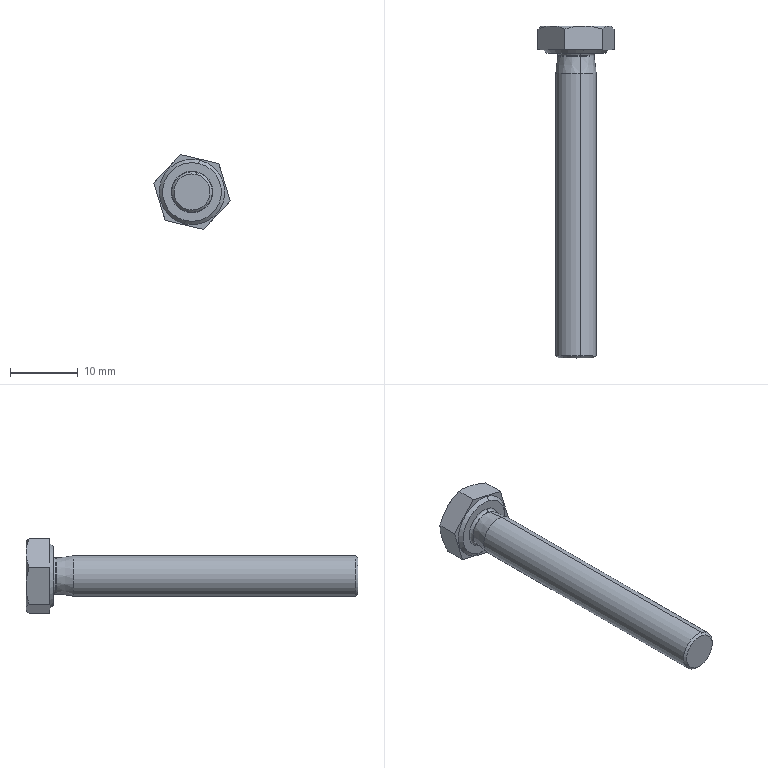Part | STEP file | Cut-Revolve 2-16 | 1 solid | 28 faces | box 11.242 x 49 x 11.054 mm | volume 1597 mm3 | cone 12 | plane 10 | torus 4 | cylinder 2 | commonest cylinder face diameters 6 x2
STEP:
#1=CARTESIAN_POINT('',(-1488.127,1719.714,2889.355));
#2=VERTEX_POINT('',#1);
#3=CARTESIAN_POINT('',(-1488.036,1720.114,2889.745));
#4=VERTEX_POINT('',#3);
#5=CARTESIAN_POINT('',(-1488.036,1719.714,2889.745));
#6=DIRECTION('',(0.9736,0.,-0.2284));
#7=DIRECTION('',(-0.2284,0.,-0.9736));
#8=AXIS2_PLACEMENT_3D('',#5,#6,#7);
#9=CIRCLE('',#8,0.4);
#10=EDGE_CURVE('',#2,#4,#9,.T.);
#11=ORIENTED_EDGE('',*,*,#10,.F.);
#12=CARTESIAN_POINT('',(-1489.349,1719.714,2884.146));
#13=VERTEX_POINT('',#12);
#14=CARTESIAN_POINT('',(-1488.738,1719.714,2886.751));
#15=DIRECTION('',(0.,1.,0.));
#16=DIRECTION('',(0.2284,0.,0.9736));
#17=AXIS2_PLACEMENT_3D('',#14,#15,#16);
#18=CIRCLE('',#17,2.675);
#19=EDGE_CURVE('',#2,#13,#18,.T.);
#20=ORIENTED_EDGE('',*,*,#19,.T.);
#21=CARTESIAN_POINT('',(-1489.441,1720.114,2883.757));
#22=VERTEX_POINT('',#21);
#23=CARTESIAN_POINT('',(-1489.441,1719.714,2883.757));
#24=DIRECTION('',(-0.9736,0.,0.2284));
#25=DIRECTION('',(0.2284,0.,0.9736));
#26=AXIS2_PLACEMENT_3D('',#23,#24,#25);
#27=CIRCLE('',#26,0.4);
#28=EDGE_CURVE('',#13,#22,#27,.T.);
#29=ORIENTED_EDGE('',*,*,#28,.T.);
#30=CARTESIAN_POINT('',(-1488.738,1720.114,2886.751));
#31=DIRECTION('',(0.,1.,0.));
#32=DIRECTION('',(0.2284,0.,0.9736));
#33=AXIS2_PLACEMENT_3D('',#30,#31,#32);
#34=CIRCLE('',#33,3.075);
#35=EDGE_CURVE('',#4,#22,#34,.T.);
#36=ORIENTED_EDGE('',*,*,#35,.F.);
#37=EDGE_LOOP('',(#11,#20,#29,#36));
#38=FACE_OUTER_BOUND('',#37,.T.);
#39=CARTESIAN_POINT('',(-1488.738,1719.714,2886.751));
#40=DIRECTION('',(0.,1.,0.));
#41=DIRECTION('',(-0.2284,0.,-0.9736));
#42=AXIS2_PLACEMENT_3D('',#39,#40,#41);
#43=TOROIDAL_SURFACE('',#42,3.075,0.4);
#44=ADVANCED_FACE('',(#38),#43,.F.);
#45=ORIENTED_EDGE('',*,*,#28,.F.);
#46=CARTESIAN_POINT('',(-1488.738,1719.714,2886.751));
#47=DIRECTION('',(0.,1.,0.));
#48=DIRECTION('',(0.2284,0.,0.9736));
#49=AXIS2_PLACEMENT_3D('',#46,#47,#48);
#50=CIRCLE('',#49,2.675);
#51=EDGE_CURVE('',#13,#2,#50,.T.);
#52=ORIENTED_EDGE('',*,*,#51,.T.);
#53=ORIENTED_EDGE('',*,*,#10,.T.);
#54=CARTESIAN_POINT('',(-1488.738,1720.114,2886.751));
#55=DIRECTION('',(0.,1.,0.));
#56=DIRECTION('',(0.2284,0.,0.9736));
#57=AXIS2_PLACEMENT_3D('',#54,#55,#56);
#58=CIRCLE('',#57,3.075);
#59=EDGE_CURVE('',#22,#4,#58,.T.);
#60=ORIENTED_EDGE('',*,*,#59,.F.);
#61=EDGE_LOOP('',(#45,#52,#53,#60));
#62=FACE_OUTER_BOUND('',#61,.T.);
#63=CARTESIAN_POINT('',(-1488.738,1719.714,2886.751));
#64=DIRECTION('',(0.,1.,0.));
#65=DIRECTION('',(-0.2284,0.,-0.9736));
#66=AXIS2_PLACEMENT_3D('',#63,#64,#65);
#67=TOROIDAL_SURFACE('',#66,3.075,0.4);
#68=ADVANCED_FACE('',(#62),#67,.F.);
#69=CARTESIAN_POINT('',(-1487.747,1720.114,2890.976));
#70=VERTEX_POINT('',#69);
#71=CARTESIAN_POINT('',(-1489.73,1720.114,2882.525));
#72=VERTEX_POINT('',#71);
#73=CARTESIAN_POINT('',(-1488.738,1720.114,2886.751));
#74=DIRECTION('',(0.,1.,0.));
#75=DIRECTION('',(0.2284,0.,0.9736));
#76=AXIS2_PLACEMENT_3D('',#73,#74,#75);
#77=CIRCLE('',#76,4.34);
#78=EDGE_CURVE('',#70,#72,#77,.T.);
#79=ORIENTED_EDGE('',*,*,#78,.T.);
#80=CARTESIAN_POINT('',(-1489.844,1720.614,2882.039));
#81=VERTEX_POINT('',#80);
#82=CARTESIAN_POINT('',(-1489.844,1720.614,2882.039));
#83=DIRECTION('',(-0.1615,0.7071,-0.6884));
#84=VECTOR('',#83,1000.);
#85=LINE('',#82,#84);
#86=EDGE_CURVE('',#72,#81,#85,.T.);
#87=ORIENTED_EDGE('',*,*,#86,.T.);
#88=CARTESIAN_POINT('',(-1487.633,1720.614,2891.463));
#89=VERTEX_POINT('',#88);
#90=CARTESIAN_POINT('',(-1488.738,1720.614,2886.751));
#91=DIRECTION('',(0.,1.,0.));
#92=DIRECTION('',(0.2284,0.,0.9736));
#93=AXIS2_PLACEMENT_3D('',#90,#91,#92);
#94=CIRCLE('',#93,4.84);
#95=EDGE_CURVE('',#89,#81,#94,.T.);
#96=ORIENTED_EDGE('',*,*,#95,.F.);
#97=CARTESIAN_POINT('',(-1487.633,1720.614,2891.463));
#98=DIRECTION('',(0.1615,0.7071,0.6884));
#99=VECTOR('',#98,1000.);
#100=LINE('',#97,#99);
#101=EDGE_CURVE('',#70,#89,#100,.T.);
#102=ORIENTED_EDGE('',*,*,#101,.F.);
#103=EDGE_LOOP('',(#79,#87,#96,#102));
#104=FACE_OUTER_BOUND('',#103,.T.);
#105=CARTESIAN_POINT('',(-1488.738,1720.614,2886.751));
#106=DIRECTION('',(0.,1.,0.));
#107=DIRECTION('',(-0.2284,0.,-0.9736));
#108=AXIS2_PLACEMENT_3D('',#105,#106,#107);
#109=CONICAL_SURFACE('',#108,4.84,0.7854);
#110=ADVANCED_FACE('',(#104),#109,.T.);
#111=CARTESIAN_POINT('',(-1489.347,1675.114,2884.155));
#112=VERTEX_POINT('',#111);
#113=CARTESIAN_POINT('',(-1488.129,1675.114,2889.347));
#114=VERTEX_POINT('',#113);
#115=CARTESIAN_POINT('',(-1488.738,1675.114,2886.751));
#116=DIRECTION('',(0.,-1.,0.));
#117=DIRECTION('',(0.2284,0.,0.9736));
#118=AXIS2_PLACEMENT_3D('',#115,#116,#117);
#119=CIRCLE('',#118,2.667);
#120=EDGE_CURVE('',#112,#114,#119,.T.);
#121=ORIENTED_EDGE('',*,*,#120,.F.);
#122=CARTESIAN_POINT('',(-1489.423,1675.448,2883.83));
#123=VERTEX_POINT('',#122);
#124=CARTESIAN_POINT('',(-1489.423,1675.448,2883.83));
#125=DIRECTION('',(-0.1615,0.7071,-0.6884));
#126=VECTOR('',#125,1000.);
#127=LINE('',#124,#126);
#128=EDGE_CURVE('',#112,#123,#127,.T.);
#129=ORIENTED_EDGE('',*,*,#128,.T.);
#130=CARTESIAN_POINT('',(-1488.053,1675.448,2889.671));
#131=VERTEX_POINT('',#130);
#132=CARTESIAN_POINT('',(-1488.738,1675.448,2886.751));
#133=DIRECTION('',(0.,1.,0.));
#134=DIRECTION('',(0.2284,0.,0.9736));
#135=AXIS2_PLACEMENT_3D('',#132,#133,#134);
#136=CIRCLE('',#135,3.);
#137=EDGE_CURVE('',#131,#123,#136,.T.);
#138=ORIENTED_EDGE('',*,*,#137,.F.);
#139=CARTESIAN_POINT('',(-1488.053,1675.448,2889.671));
#140=DIRECTION('',(0.1615,0.7071,0.6884));
#141=VECTOR('',#140,1000.);
#142=LINE('',#139,#141);
#143=EDGE_CURVE('',#114,#131,#142,.T.);
#144=ORIENTED_EDGE('',*,*,#143,.F.);
#145=EDGE_LOOP('',(#121,#129,#138,#144));
#146=FACE_OUTER_BOUND('',#145,.T.);
#147=CARTESIAN_POINT('',(-1488.738,1675.448,2886.751));
#148=DIRECTION('',(0.,1.,0.));
#149=DIRECTION('',(-0.2284,0.,-0.9736));
#150=AXIS2_PLACEMENT_3D('',#147,#148,#149);
#151=CONICAL_SURFACE('',#150,3.,0.7854);
#152=ADVANCED_FACE('',(#146),#151,.T.);
#153=ORIENTED_EDGE('',*,*,#51,.F.);
#154=CARTESIAN_POINT('',(-1489.35,1719.664,2884.143));
#155=VERTEX_POINT('',#154);
#156=CARTESIAN_POINT('',(-1489.441,1719.714,2883.757));
#157=DIRECTION('',(0.9736,0.,-0.2284));
#158=DIRECTION('',(0.2284,0.,0.9736));
#159=AXIS2_PLACEMENT_3D('',#156,#157,#158);
#160=CIRCLE('',#159,0.4);
#161=EDGE_CURVE('',#13,#155,#160,.T.);
#162=ORIENTED_EDGE('',*,*,#161,.T.);
#163=CARTESIAN_POINT('',(-1488.127,1719.664,2889.358));
#164=VERTEX_POINT('',#163);
#165=CARTESIAN_POINT('',(-1488.738,1719.664,2886.751));
#166=DIRECTION('',(0.,1.,0.));
#167=DIRECTION('',(0.2284,0.,0.9736));
#168=AXIS2_PLACEMENT_3D('',#165,#166,#167);
#169=CIRCLE('',#168,2.678);
#170=EDGE_CURVE('',#155,#164,#169,.T.);
#171=ORIENTED_EDGE('',*,*,#170,.T.);
#172=CARTESIAN_POINT('',(-1488.036,1719.714,2889.745));
#173=DIRECTION('',(-0.9736,0.,0.2284));
#174=DIRECTION('',(-0.2284,0.,-0.9736));
#175=AXIS2_PLACEMENT_3D('',#172,#173,#174);
#176=CIRCLE('',#175,0.4);
#177=EDGE_CURVE('',#2,#164,#176,.T.);
#178=ORIENTED_EDGE('',*,*,#177,.F.);
#179=EDGE_LOOP('',(#153,#162,#171,#178));
#180=FACE_OUTER_BOUND('',#179,.T.);
#181=CARTESIAN_POINT('',(-1488.738,1719.714,2886.751));
#182=DIRECTION('',(0.,1.,0.));
#183=DIRECTION('',(-0.2284,0.,-0.9736));
#184=AXIS2_PLACEMENT_3D('',#181,#182,#183);
#185=TOROIDAL_SURFACE('',#184,3.075,0.4);
#186=ADVANCED_FACE('',(#180),#185,.F.);
#187=ORIENTED_EDGE('',*,*,#137,.T.);
#188=CARTESIAN_POINT('',(-1489.423,1717.114,2883.83));
#189=VERTEX_POINT('',#188);
#190=CARTESIAN_POINT('',(-1489.423,1720.114,2883.83));
#191=DIRECTION('',(0.,1.,0.));
#192=VECTOR('',#191,1000.);
#193=LINE('',#190,#192);
#194=EDGE_CURVE('',#123,#189,#193,.T.);
#195=ORIENTED_EDGE('',*,*,#194,.T.);
#196=CARTESIAN_POINT('',(-1488.053,1717.114,2889.671));
#197=VERTEX_POINT('',#196);
#198=CARTESIAN_POINT('',(-1488.738,1717.114,2886.751));
#199=DIRECTION('',(0.,1.,0.));
#200=DIRECTION('',(0.2284,0.,0.9736));
#201=AXIS2_PLACEMENT_3D('',#198,#199,#200);
#202=CIRCLE('',#201,3.);
#203=EDGE_CURVE('',#197,#189,#202,.T.);
#204=ORIENTED_EDGE('',*,*,#203,.F.);
#205=CARTESIAN_POINT('',(-1488.053,1720.114,2889.671));
#206=DIRECTION('',(0.,1.,0.));
#207=VECTOR('',#206,1000.);
#208=LINE('',#205,#207);
#209=EDGE_CURVE('',#131,#197,#208,.T.);
#210=ORIENTED_EDGE('',*,*,#209,.F.);
#211=EDGE_LOOP('',(#187,#195,#204,#210));
#212=FACE_OUTER_BOUND('',#211,.T.);
#213=CARTESIAN_POINT('',(-1488.738,1720.114,2886.751));
#214=DIRECTION('',(0.,1.,0.));
#215=DIRECTION('',(-0.2284,0.,-0.9736));
#216=AXIS2_PLACEMENT_3D('',#213,#214,#215);
#217=CYLINDRICAL_SURFACE('',#216,3.);
#218=ADVANCED_FACE('',(#212),#217,.T.);
#219=CARTESIAN_POINT('',(-1488.738,1719.664,2886.751));
#220=DIRECTION('',(0.,1.,0.));
#221=DIRECTION('',(0.2284,0.,0.9736));
#222=AXIS2_PLACEMENT_3D('',#219,#220,#221);
#223=CIRCLE('',#222,2.678);
#224=EDGE_CURVE('',#164,#155,#223,.T.);
#225=ORIENTED_EDGE('',*,*,#224,.F.);
#226=CARTESIAN_POINT('',(-1488.053,1717.114,2889.671));
#227=DIRECTION('',(-0.02858,0.9921,-0.1218));
#228=VECTOR('',#227,1000.);
#229=LINE('',#226,#228);
#230=EDGE_CURVE('',#197,#164,#229,.T.);
#231=ORIENTED_EDGE('',*,*,#230,.F.);
#232=ORIENTED_EDGE('',*,*,#203,.T.);
#233=CARTESIAN_POINT('',(-1489.423,1717.114,2883.83));
#234=DIRECTION('',(0.02858,0.9921,0.1218));
#235=VECTOR('',#234,1000.);
#236=LINE('',#233,#235);
#237=EDGE_CURVE('',#189,#155,#236,.T.);
#238=ORIENTED_EDGE('',*,*,#237,.T.);
#239=EDGE_LOOP('',(#225,#231,#232,#238));
#240=FACE_OUTER_BOUND('',#239,.T.);
#241=CARTESIAN_POINT('',(-1488.738,1717.114,2886.751));
#242=DIRECTION('',(0.,-1.,0.));
#243=DIRECTION('',(0.2284,0.,0.9736));
#244=AXIS2_PLACEMENT_3D('',#241,#242,#243);
#245=CONICAL_SURFACE('',#244,3.,0.1255);
#246=ADVANCED_FACE('',(#240),#245,.T.);
#247=ORIENTED_EDGE('',*,*,#35,.T.);
#248=ORIENTED_EDGE('',*,*,#59,.T.);
#249=EDGE_LOOP('',(#247,#248));
#250=FACE_BOUND('',#249,.T.);
#251=ORIENTED_EDGE('',*,*,#78,.F.);
#252=CARTESIAN_POINT('',(-1488.738,1720.114,2886.751));
#253=DIRECTION('',(0.,1.,0.));
#254=DIRECTION('',(0.2284,0.,0.9736));
#255=AXIS2_PLACEMENT_3D('',#252,#253,#254);
#256=CIRCLE('',#255,4.34);
#257=EDGE_CURVE('',#72,#70,#256,.T.);
#258=ORIENTED_EDGE('',*,*,#257,.F.);
#259=EDGE_LOOP('',(#251,#258));
#260=FACE_OUTER_BOUND('',#259,.T.);
#261=CARTESIAN_POINT('',(-1487.07,1720.114,2881.224));
#262=DIRECTION('',(0.,-1.,0.));
#263=DIRECTION('',(0.2284,0.,0.9736));
#264=AXIS2_PLACEMENT_3D('',#261,#262,#263);
#265=PLANE('',#264);
#266=ADVANCED_FACE('',(#250,#260),#265,.T.);
#267=ORIENTED_EDGE('',*,*,#230,.T.);
#268=ORIENTED_EDGE('',*,*,#170,.F.);
#269=ORIENTED_EDGE('',*,*,#237,.F.);
#270=CARTESIAN_POINT('',(-1488.738,1717.114,2886.751));
#271=DIRECTION('',(0.,1.,0.));
#272=DIRECTION('',(0.2284,0.,0.9736));
#273=AXIS2_PLACEMENT_3D('',#270,#271,#272);
#274=CIRCLE('',#273,3.);
#275=EDGE_CURVE('',#189,#197,#274,.T.);
#276=ORIENTED_EDGE('',*,*,#275,.T.);
#277=EDGE_LOOP('',(#267,#268,#269,#276));
#278=FACE_OUTER_BOUND('',#277,.T.);
#279=CARTESIAN_POINT('',(-1488.738,1717.114,2886.751));
#280=DIRECTION('',(0.,-1.,0.));
#281=DIRECTION('',(0.2284,0.,0.9736));
#282=AXIS2_PLACEMENT_3D('',#279,#280,#281);
#283=CONICAL_SURFACE('',#282,3.,0.1255);
#284=ADVANCED_FACE('',(#278),#283,.T.);
#285=ORIENTED_EDGE('',*,*,#194,.F.);
#286=CARTESIAN_POINT('',(-1488.738,1675.448,2886.751));
#287=DIRECTION('',(0.,1.,0.));
#288=DIRECTION('',(0.2284,0.,0.9736));
#289=AXIS2_PLACEMENT_3D('',#286,#287,#288);
#290=CIRCLE('',#289,3.);
#291=EDGE_CURVE('',#123,#131,#290,.T.);
#292=ORIENTED_EDGE('',*,*,#291,.T.);
#293=ORIENTED_EDGE('',*,*,#209,.T.);
#294=ORIENTED_EDGE('',*,*,#275,.F.);
#295=EDGE_LOOP('',(#285,#292,#293,#294));
#296=FACE_OUTER_BOUND('',#295,.T.);
#297=CARTESIAN_POINT('',(-1488.738,1720.114,2886.751));
#298=DIRECTION('',(0.,1.,0.));
#299=DIRECTION('',(-0.2284,0.,-0.9736));
#300=AXIS2_PLACEMENT_3D('',#297,#298,#299);
#301=CYLINDRICAL_SURFACE('',#300,3.);
#302=ADVANCED_FACE('',(#296),#301,.T.);
#303=CARTESIAN_POINT('',(-1488.738,1675.114,2886.751));
#304=DIRECTION('',(0.,-1.,0.));
#305=DIRECTION('',(0.2284,0.,0.9736));
#306=AXIS2_PLACEMENT_3D('',#303,#304,#305);
#307=CIRCLE('',#306,2.667);
#308=EDGE_CURVE('',#114,#112,#307,.T.);
#309=ORIENTED_EDGE('',*,*,#308,.T.);
#310=ORIENTED_EDGE('',*,*,#120,.T.);
#311=EDGE_LOOP('',(#309,#310));
#312=FACE_OUTER_BOUND('',#311,.T.);
#313=CARTESIAN_POINT('',(-1485.818,1675.114,2886.065));
#314=DIRECTION('',(0.,1.,0.));
#315=DIRECTION('',(-0.2284,0.,-0.9736));
#316=AXIS2_PLACEMENT_3D('',#313,#314,#315);
#317=PLANE('',#316);
#318=ADVANCED_FACE('',(#312),#317,.F.);
#319=ORIENTED_EDGE('',*,*,#19,.F.);
#320=ORIENTED_EDGE('',*,*,#177,.T.);
#321=ORIENTED_EDGE('',*,*,#224,.T.);
#322=ORIENTED_EDGE('',*,*,#161,.F.);
#323=EDGE_LOOP('',(#319,#320,#321,#322));
#324=FACE_OUTER_BOUND('',#323,.T.);
#325=CARTESIAN_POINT('',(-1488.738,1719.714,2886.751));
#326=DIRECTION('',(0.,1.,0.));
#327=DIRECTION('',(-0.2284,0.,-0.9736));
#328=AXIS2_PLACEMENT_3D('',#325,#326,#327);
#329=TOROIDAL_SURFACE('',#328,3.075,0.4);
#330=ADVANCED_FACE('',(#324),#329,.F.);
#331=ORIENTED_EDGE('',*,*,#128,.F.);
#332=ORIENTED_EDGE('',*,*,#308,.F.);
#333=ORIENTED_EDGE('',*,*,#143,.T.);
#334=ORIENTED_EDGE('',*,*,#291,.F.);
#335=EDGE_LOOP('',(#331,#332,#333,#334));
#336=FACE_OUTER_BOUND('',#335,.T.);
#337=CARTESIAN_POINT('',(-1488.738,1675.448,2886.751));
#338=DIRECTION('',(0.,1.,0.));
#339=DIRECTION('',(-0.2284,0.,-0.9736));
#340=AXIS2_PLACEMENT_3D('',#337,#338,#339);
#341=CONICAL_SURFACE('',#340,3.,0.7854);
#342=ADVANCED_FACE('',(#336),#341,.T.);
#343=ORIENTED_EDGE('',*,*,#95,.T.);
#344=CARTESIAN_POINT('',(-1488.738,1720.614,2886.751));
#345=DIRECTION('',(0.,1.,0.));
#346=DIRECTION('',(0.2284,0.,0.9736));
#347=AXIS2_PLACEMENT_3D('',#344,#345,#346);
#348=CIRCLE('',#347,4.84);
#349=EDGE_CURVE('',#81,#89,#348,.T.);
#350=ORIENTED_EDGE('',*,*,#349,.T.);
#351=EDGE_LOOP('',(#343,#350));
#352=FACE_BOUND('',#351,.T.);
#353=CARTESIAN_POINT('',(-1492.691,1720.614,2882.542));
#354=VERTEX_POINT('',#353);
#355=CARTESIAN_POINT('',(-1487.07,1720.614,2881.224));
#356=VERTEX_POINT('',#355);
#357=CARTESIAN_POINT('',(-1492.691,1720.614,2882.542));
#358=DIRECTION('',(0.9736,0.,-0.2284));
#359=VECTOR('',#358,1000.);
#360=LINE('',#357,#359);
#361=EDGE_CURVE('',#354,#356,#360,.T.);
#362=ORIENTED_EDGE('',*,*,#361,.T.);
#363=CARTESIAN_POINT('',(-1483.117,1720.614,2885.432));
#364=VERTEX_POINT('',#363);
#365=CARTESIAN_POINT('',(-1487.07,1720.614,2881.224));
#366=DIRECTION('',(0.6846,0.,0.7289));
#367=VECTOR('',#366,1000.);
#368=LINE('',#365,#367);
#369=EDGE_CURVE('',#356,#364,#368,.T.);
#370=ORIENTED_EDGE('',*,*,#369,.T.);
#371=CARTESIAN_POINT('',(-1484.786,1720.614,2890.959));
#372=VERTEX_POINT('',#371);
#373=CARTESIAN_POINT('',(-1483.117,1720.614,2885.432));
#374=DIRECTION('',(-0.289,0.,0.9573));
#375=VECTOR('',#374,1000.);
#376=LINE('',#373,#375);
#377=EDGE_CURVE('',#364,#372,#376,.T.);
#378=ORIENTED_EDGE('',*,*,#377,.T.);
#379=CARTESIAN_POINT('',(-1490.407,1720.614,2892.278));
#380=VERTEX_POINT('',#379);
#381=CARTESIAN_POINT('',(-1484.786,1720.614,2890.959));
#382=DIRECTION('',(-0.9736,0.,0.2284));
#383=VECTOR('',#382,1000.);
#384=LINE('',#381,#383);
#385=EDGE_CURVE('',#372,#380,#384,.T.);
#386=ORIENTED_EDGE('',*,*,#385,.T.);
#387=CARTESIAN_POINT('',(-1494.359,1720.614,2888.069));
#388=VERTEX_POINT('',#387);
#389=CARTESIAN_POINT('',(-1490.407,1720.614,2892.278));
#390=DIRECTION('',(-0.6846,0.,-0.7289));
#391=VECTOR('',#390,1000.);
#392=LINE('',#389,#391);
#393=EDGE_CURVE('',#380,#388,#392,.T.);
#394=ORIENTED_EDGE('',*,*,#393,.T.);
#395=CARTESIAN_POINT('',(-1494.359,1720.614,2888.069));
#396=DIRECTION('',(0.289,0.,-0.9573));
#397=VECTOR('',#396,1000.);
#398=LINE('',#395,#397);
#399=EDGE_CURVE('',#388,#354,#398,.T.);
#400=ORIENTED_EDGE('',*,*,#399,.T.);
#401=EDGE_LOOP('',(#362,#370,#378,#386,#394,#400));
#402=FACE_OUTER_BOUND('',#401,.T.);
#403=CARTESIAN_POINT('',(-1493.45,1720.614,2887.856));
#404=DIRECTION('',(0.,-1.,0.));
#405=DIRECTION('',(0.2284,0.,0.9736));
#406=AXIS2_PLACEMENT_3D('',#403,#404,#405);
#407=PLANE('',#406);
#408=ADVANCED_FACE('',(#352,#402),#407,.T.);
#409=ORIENTED_EDGE('',*,*,#86,.F.);
#410=ORIENTED_EDGE('',*,*,#257,.T.);
#411=ORIENTED_EDGE('',*,*,#101,.T.);
#412=ORIENTED_EDGE('',*,*,#349,.F.);
#413=EDGE_LOOP('',(#409,#410,#411,#412));
#414=FACE_OUTER_BOUND('',#413,.T.);
#415=CARTESIAN_POINT('',(-1488.738,1720.614,2886.751));
#416=DIRECTION('',(0.,1.,0.));
#417=DIRECTION('',(-0.2284,0.,-0.9736));
#418=AXIS2_PLACEMENT_3D('',#415,#416,#417);
#419=CONICAL_SURFACE('',#418,4.84,0.7854);
#420=ADVANCED_FACE('',(#414),#419,.T.);
#421=CARTESIAN_POINT('',(-1489.88,1724.114,2881.883));
#422=VERTEX_POINT('',#421);
#423=CARTESIAN_POINT('',(-1485.094,1724.114,2883.328));
#424=VERTEX_POINT('',#423);
#425=CARTESIAN_POINT('',(-1488.738,1724.114,2886.751));
#426=DIRECTION('',(0.,-1.,0.));
#427=DIRECTION('',(-0.2284,0.,-0.9736));
#428=AXIS2_PLACEMENT_3D('',#425,#426,#427);
#429=CIRCLE('',#428,5.);
#430=EDGE_CURVE('',#422,#424,#429,.T.);
#431=ORIENTED_EDGE('',*,*,#430,.F.);
#432=CARTESIAN_POINT('',(-1493.525,1724.114,2885.306));
#433=VERTEX_POINT('',#432);
#434=CARTESIAN_POINT('',(-1488.738,1724.114,2886.751));
#435=DIRECTION('',(0.,-1.,0.));
#436=DIRECTION('',(-0.2284,0.,-0.9736));
#437=AXIS2_PLACEMENT_3D('',#434,#435,#436);
#438=CIRCLE('',#437,5.);
#439=EDGE_CURVE('',#433,#422,#438,.T.);
#440=ORIENTED_EDGE('',*,*,#439,.F.);
#441=CARTESIAN_POINT('',(-1492.383,1724.114,2890.174));
#442=VERTEX_POINT('',#441);
#443=CARTESIAN_POINT('',(-1488.738,1724.114,2886.751));
#444=DIRECTION('',(0.,-1.,0.));
#445=DIRECTION('',(-0.2284,0.,-0.9736));
#446=AXIS2_PLACEMENT_3D('',#443,#444,#445);
#447=CIRCLE('',#446,5.);
#448=EDGE_CURVE('',#442,#433,#447,.T.);
#449=ORIENTED_EDGE('',*,*,#448,.F.);
#450=CARTESIAN_POINT('',(-1487.596,1724.114,2891.619));
#451=VERTEX_POINT('',#450);
#452=CARTESIAN_POINT('',(-1488.738,1724.114,2886.751));
#453=DIRECTION('',(0.,-1.,0.));
#454=DIRECTION('',(-0.2284,0.,-0.9736));
#455=AXIS2_PLACEMENT_3D('',#452,#453,#454);
#456=CIRCLE('',#455,5.);
#457=EDGE_CURVE('',#451,#442,#456,.T.);
#458=ORIENTED_EDGE('',*,*,#457,.F.);
#459=CARTESIAN_POINT('',(-1483.952,1724.114,2888.196));
#460=VERTEX_POINT('',#459);
#461=CARTESIAN_POINT('',(-1488.738,1724.114,2886.751));
#462=DIRECTION('',(0.,1.,0.));
#463=DIRECTION('',(0.2284,0.,0.9736));
#464=AXIS2_PLACEMENT_3D('',#461,#462,#463);
#465=CIRCLE('',#464,5.);
#466=EDGE_CURVE('',#451,#460,#465,.T.);
#467=ORIENTED_EDGE('',*,*,#466,.T.);
#468=CARTESIAN_POINT('',(-1488.738,1724.114,2886.751));
#469=DIRECTION('',(0.,-1.,0.));
#470=DIRECTION('',(-0.2284,0.,-0.9736));
#471=AXIS2_PLACEMENT_3D('',#468,#469,#470);
#472=CIRCLE('',#471,5.);
#473=EDGE_CURVE('',#424,#460,#472,.T.);
#474=ORIENTED_EDGE('',*,*,#473,.F.);
#475=EDGE_LOOP('',(#431,#440,#449,#458,#467,#474));
#476=FACE_OUTER_BOUND('',#475,.T.);
#477=CARTESIAN_POINT('',(-1487.07,1724.114,2881.224));
#478=DIRECTION('',(0.,-1.,0.));
#479=DIRECTION('',(0.2284,0.,0.9736));
#480=AXIS2_PLACEMENT_3D('',#477,#478,#479);
#481=PLANE('',#480);
#482=ADVANCED_FACE('',(#476),#481,.F.);
#483=CARTESIAN_POINT('',(-1487.07,1723.668,2881.224));
#484=VERTEX_POINT('',#483);
#485=CARTESIAN_POINT('',(-1485.094,1724.114,2883.328));
#486=CARTESIAN_POINT('',(-1485.768,1724.114,2882.61));
#487=CARTESIAN_POINT('',(-1486.424,1723.94,2881.911));
#488=CARTESIAN_POINT('',(-1487.07,1723.668,2881.224));
#489=B_SPLINE_CURVE_WITH_KNOTS('',3,(#485,#486,#487,#488),.UNSPECIFIED.,.F.,.F.,(4,4),(0.,0.002921),.UNSPECIFIED.);
#490=EDGE_CURVE('',#424,#484,#489,.T.);
#491=ORIENTED_EDGE('',*,*,#490,.T.);
#492=CARTESIAN_POINT('',(-1487.07,1723.668,2881.224));
#493=CARTESIAN_POINT('',(-1487.988,1723.94,2881.439));
#494=CARTESIAN_POINT('',(-1488.921,1724.114,2881.658));
#495=CARTESIAN_POINT('',(-1489.88,1724.114,2881.883));
#496=B_SPLINE_CURVE_WITH_KNOTS('',3,(#492,#493,#494,#495),.UNSPECIFIED.,.F.,.F.,(4,4),(0.,0.002921),.UNSPECIFIED.);
#497=EDGE_CURVE('',#484,#422,#496,.T.);
#498=ORIENTED_EDGE('',*,*,#497,.T.);
#499=ORIENTED_EDGE('',*,*,#430,.T.);
#500=EDGE_LOOP('',(#491,#498,#499));
#501=FACE_OUTER_BOUND('',#500,.T.);
#502=CARTESIAN_POINT('',(-1488.738,1724.114,2886.751));
#503=DIRECTION('',(0.,-1.,0.));
#504=DIRECTION('',(-0.2284,0.,-0.9736));
#505=AXIS2_PLACEMENT_3D('',#502,#503,#504);
#506=CONICAL_SURFACE('',#505,5.,1.047);
#507=ADVANCED_FACE('',(#501),#506,.T.);
#508=CARTESIAN_POINT('',(-1483.117,1723.668,2885.432));
#509=VERTEX_POINT('',#508);
#510=CARTESIAN_POINT('',(-1483.952,1724.114,2888.196));
#511=CARTESIAN_POINT('',(-1483.667,1724.114,2887.252));
#512=CARTESIAN_POINT('',(-1483.39,1723.94,2886.335));
#513=CARTESIAN_POINT('',(-1483.117,1723.668,2885.432));
#514=B_SPLINE_CURVE_WITH_KNOTS('',3,(#510,#511,#512,#513),.UNSPECIFIED.,.F.,.F.,(4,4),(0.,0.002921),.UNSPECIFIED.);
#515=EDGE_CURVE('',#460,#509,#514,.T.);
#516=ORIENTED_EDGE('',*,*,#515,.T.);
#517=CARTESIAN_POINT('',(-1483.117,1723.668,2885.432));
#518=CARTESIAN_POINT('',(-1483.763,1723.94,2884.745));
#519=CARTESIAN_POINT('',(-1484.419,1724.114,2884.046));
#520=CARTESIAN_POINT('',(-1485.094,1724.114,2883.328));
#521=B_SPLINE_CURVE_WITH_KNOTS('',3,(#517,#518,#519,#520),.UNSPECIFIED.,.F.,.F.,(4,4),(0.,0.002921),.UNSPECIFIED.);
#522=EDGE_CURVE('',#509,#424,#521,.T.);
#523=ORIENTED_EDGE('',*,*,#522,.T.);
#524=ORIENTED_EDGE('',*,*,#473,.T.);
#525=EDGE_LOOP('',(#516,#523,#524));
#526=FACE_OUTER_BOUND('',#525,.T.);
#527=CARTESIAN_POINT('',(-1488.738,1724.114,2886.751));
#528=DIRECTION('',(0.,-1.,0.));
#529=DIRECTION('',(-0.2284,0.,-0.9736));
#530=AXIS2_PLACEMENT_3D('',#527,#528,#529);
#531=CONICAL_SURFACE('',#530,5.,1.047);
#532=ADVANCED_FACE('',(#526),#531,.T.);
#533=CARTESIAN_POINT('',(-1484.786,1723.668,2890.959));
#534=VERTEX_POINT('',#533);
#535=CARTESIAN_POINT('',(-1484.786,1723.668,2890.959));
#536=CARTESIAN_POINT('',(-1484.513,1723.94,2890.056));
#537=CARTESIAN_POINT('',(-1484.236,1724.114,2889.139));
#538=CARTESIAN_POINT('',(-1483.952,1724.114,2888.196));
#539=B_SPLINE_CURVE_WITH_KNOTS('',3,(#535,#536,#537,#538),.UNSPECIFIED.,.F.,.F.,(4,4),(0.,0.002921),.UNSPECIFIED.);
#540=EDGE_CURVE('',#534,#460,#539,.T.);
#541=ORIENTED_EDGE('',*,*,#540,.T.);
#542=ORIENTED_EDGE('',*,*,#466,.F.);
#543=CARTESIAN_POINT('',(-1487.596,1724.114,2891.619));
#544=CARTESIAN_POINT('',(-1486.637,1724.114,2891.393));
#545=CARTESIAN_POINT('',(-1485.704,1723.94,2891.175));
#546=CARTESIAN_POINT('',(-1484.786,1723.668,2890.959));
#547=B_SPLINE_CURVE_WITH_KNOTS('',3,(#543,#544,#545,#546),.UNSPECIFIED.,.F.,.F.,(4,4),(0.,0.002921),.UNSPECIFIED.);
#548=EDGE_CURVE('',#451,#534,#547,.T.);
#549=ORIENTED_EDGE('',*,*,#548,.T.);
#550=EDGE_LOOP('',(#541,#542,#549));
#551=FACE_OUTER_BOUND('',#550,.T.);
#552=CARTESIAN_POINT('',(-1488.738,1724.114,2886.751));
#553=DIRECTION('',(0.,-1.,0.));
#554=DIRECTION('',(-0.2284,0.,-0.9736));
#555=AXIS2_PLACEMENT_3D('',#552,#553,#554);
#556=CONICAL_SURFACE('',#555,5.,1.047);
#557=ADVANCED_FACE('',(#551),#556,.T.);
#558=CARTESIAN_POINT('',(-1490.407,1723.668,2892.278));
#559=VERTEX_POINT('',#558);
#560=CARTESIAN_POINT('',(-1490.407,1723.668,2892.278));
#561=CARTESIAN_POINT('',(-1489.488,1723.94,2892.062));
#562=CARTESIAN_POINT('',(-1488.555,1724.114,2891.844));
#563=CARTESIAN_POINT('',(-1487.596,1724.114,2891.619));
#564=B_SPLINE_CURVE_WITH_KNOTS('',3,(#560,#561,#562,#563),.UNSPECIFIED.,.F.,.F.,(4,4),(0.,0.002921),.UNSPECIFIED.);
#565=EDGE_CURVE('',#559,#451,#564,.T.);
#566=ORIENTED_EDGE('',*,*,#565,.T.);
#567=ORIENTED_EDGE('',*,*,#457,.T.);
#568=CARTESIAN_POINT('',(-1492.383,1724.114,2890.174));
#569=CARTESIAN_POINT('',(-1491.708,1724.114,2890.892));
#570=CARTESIAN_POINT('',(-1491.052,1723.94,2891.59));
#571=CARTESIAN_POINT('',(-1490.407,1723.668,2892.278));
#572=B_SPLINE_CURVE_WITH_KNOTS('',3,(#568,#569,#570,#571),.UNSPECIFIED.,.F.,.F.,(4,4),(0.,0.002921),.UNSPECIFIED.);
#573=EDGE_CURVE('',#442,#559,#572,.T.);
#574=ORIENTED_EDGE('',*,*,#573,.T.);
#575=EDGE_LOOP('',(#566,#567,#574));
#576=FACE_OUTER_BOUND('',#575,.T.);
#577=CARTESIAN_POINT('',(-1488.738,1724.114,2886.751));
#578=DIRECTION('',(0.,-1.,0.));
#579=DIRECTION('',(-0.2284,0.,-0.9736));
#580=AXIS2_PLACEMENT_3D('',#577,#578,#579);
#581=CONICAL_SURFACE('',#580,5.,1.047);
#582=ADVANCED_FACE('',(#576),#581,.T.);
#583=CARTESIAN_POINT('',(-1492.691,1723.668,2882.542));
#584=VERTEX_POINT('',#583);
#585=CARTESIAN_POINT('',(-1489.88,1724.114,2881.883));
#586=CARTESIAN_POINT('',(-1490.84,1724.114,2882.108));
#587=CARTESIAN_POINT('',(-1491.773,1723.94,2882.327));
#588=CARTESIAN_POINT('',(-1492.691,1723.668,2882.542));
#589=B_SPLINE_CURVE_WITH_KNOTS('',3,(#585,#586,#587,#588),.UNSPECIFIED.,.F.,.F.,(4,4),(0.,0.002921),.UNSPECIFIED.);
#590=EDGE_CURVE('',#422,#584,#589,.T.);
#591=ORIENTED_EDGE('',*,*,#590,.T.);
#592=CARTESIAN_POINT('',(-1492.691,1723.668,2882.542));
#593=CARTESIAN_POINT('',(-1492.963,1723.94,2883.445));
#594=CARTESIAN_POINT('',(-1493.24,1724.114,2884.363));
#595=CARTESIAN_POINT('',(-1493.525,1724.114,2885.306));
#596=B_SPLINE_CURVE_WITH_KNOTS('',3,(#592,#593,#594,#595),.UNSPECIFIED.,.F.,.F.,(4,4),(0.,0.002921),.UNSPECIFIED.);
#597=EDGE_CURVE('',#584,#433,#596,.T.);
#598=ORIENTED_EDGE('',*,*,#597,.T.);
#599=ORIENTED_EDGE('',*,*,#439,.T.);
#600=EDGE_LOOP('',(#591,#598,#599));
#601=FACE_OUTER_BOUND('',#600,.T.);
#602=CARTESIAN_POINT('',(-1488.738,1724.114,2886.751));
#603=DIRECTION('',(0.,-1.,0.));
#604=DIRECTION('',(-0.2284,0.,-0.9736));
#605=AXIS2_PLACEMENT_3D('',#602,#603,#604);
#606=CONICAL_SURFACE('',#605,5.,1.047);
#607=ADVANCED_FACE('',(#601),#606,.T.);
#608=CARTESIAN_POINT('',(-1494.359,1723.668,2888.069));
#609=VERTEX_POINT('',#608);
#610=CARTESIAN_POINT('',(-1494.359,1723.668,2888.069));
#611=CARTESIAN_POINT('',(-1493.713,1723.94,2888.757));
#612=CARTESIAN_POINT('',(-1493.057,1724.114,2889.455));
#613=CARTESIAN_POINT('',(-1492.383,1724.114,2890.174));
#614=B_SPLINE_CURVE_WITH_KNOTS('',3,(#610,#611,#612,#613),.UNSPECIFIED.,.F.,.F.,(4,4),(0.,0.002921),.UNSPECIFIED.);
#615=EDGE_CURVE('',#609,#442,#614,.T.);
#616=ORIENTED_EDGE('',*,*,#615,.T.);
#617=ORIENTED_EDGE('',*,*,#448,.T.);
#618=CARTESIAN_POINT('',(-1493.525,1724.114,2885.306));
#619=CARTESIAN_POINT('',(-1493.81,1724.114,2886.249));
#620=CARTESIAN_POINT('',(-1494.087,1723.94,2887.166));
#621=CARTESIAN_POINT('',(-1494.359,1723.668,2888.069));
#622=B_SPLINE_CURVE_WITH_KNOTS('',3,(#618,#619,#620,#621),.UNSPECIFIED.,.F.,.F.,(4,4),(0.,0.002921),.UNSPECIFIED.);
#623=EDGE_CURVE('',#433,#609,#622,.T.);
#624=ORIENTED_EDGE('',*,*,#623,.T.);
#625=EDGE_LOOP('',(#616,#617,#624));
#626=FACE_OUTER_BOUND('',#625,.T.);
#627=CARTESIAN_POINT('',(-1488.738,1724.114,2886.751));
#628=DIRECTION('',(0.,-1.,0.));
#629=DIRECTION('',(-0.2284,0.,-0.9736));
#630=AXIS2_PLACEMENT_3D('',#627,#628,#629);
#631=CONICAL_SURFACE('',#630,5.,1.047);
#632=ADVANCED_FACE('',(#626),#631,.T.);
#633=ORIENTED_EDGE('',*,*,#399,.F.);
#634=CARTESIAN_POINT('',(-1494.359,1720.114,2888.069));
#635=DIRECTION('',(0.,1.,0.));
#636=VECTOR('',#635,1000.);
#637=LINE('',#634,#636);
#638=EDGE_CURVE('',#388,#609,#637,.T.);
#639=ORIENTED_EDGE('',*,*,#638,.T.);
#640=ORIENTED_EDGE('',*,*,#623,.F.);
#641=ORIENTED_EDGE('',*,*,#597,.F.);
#642=CARTESIAN_POINT('',(-1492.691,1720.114,2882.542));
#643=DIRECTION('',(0.,1.,0.));
#644=VECTOR('',#643,1000.);
#645=LINE('',#642,#644);
#646=EDGE_CURVE('',#354,#584,#645,.T.);
#647=ORIENTED_EDGE('',*,*,#646,.F.);
#648=EDGE_LOOP('',(#633,#639,#640,#641,#647));
#649=FACE_OUTER_BOUND('',#648,.T.);
#650=CARTESIAN_POINT('',(-1494.359,1720.114,2888.069));
#651=DIRECTION('',(0.9573,0.,0.289));
#652=DIRECTION('',(0.289,0.,-0.9573));
#653=AXIS2_PLACEMENT_3D('',#650,#651,#652);
#654=PLANE('',#653);
#655=ADVANCED_FACE('',(#649),#654,.F.);
#656=ORIENTED_EDGE('',*,*,#393,.F.);
#657=CARTESIAN_POINT('',(-1490.407,1720.114,2892.278));
#658=DIRECTION('',(0.,1.,0.));
#659=VECTOR('',#658,1000.);
#660=LINE('',#657,#659);
#661=EDGE_CURVE('',#380,#559,#660,.T.);
#662=ORIENTED_EDGE('',*,*,#661,.T.);
#663=ORIENTED_EDGE('',*,*,#573,.F.);
#664=ORIENTED_EDGE('',*,*,#615,.F.);
#665=ORIENTED_EDGE('',*,*,#638,.F.);
#666=EDGE_LOOP('',(#656,#662,#663,#664,#665));
#667=FACE_OUTER_BOUND('',#666,.T.);
#668=CARTESIAN_POINT('',(-1490.407,1720.114,2892.278));
#669=DIRECTION('',(0.7289,0.,-0.6846));
#670=DIRECTION('',(-0.6846,0.,-0.7289));
#671=AXIS2_PLACEMENT_3D('',#668,#669,#670);
#672=PLANE('',#671);
#673=ADVANCED_FACE('',(#667),#672,.F.);
#674=ORIENTED_EDGE('',*,*,#385,.F.);
#675=CARTESIAN_POINT('',(-1484.786,1720.114,2890.959));
#676=DIRECTION('',(0.,1.,0.));
#677=VECTOR('',#676,1000.);
#678=LINE('',#675,#677);
#679=EDGE_CURVE('',#372,#534,#678,.T.);
#680=ORIENTED_EDGE('',*,*,#679,.T.);
#681=ORIENTED_EDGE('',*,*,#548,.F.);
#682=ORIENTED_EDGE('',*,*,#565,.F.);
#683=ORIENTED_EDGE('',*,*,#661,.F.);
#684=EDGE_LOOP('',(#674,#680,#681,#682,#683));
#685=FACE_OUTER_BOUND('',#684,.T.);
#686=CARTESIAN_POINT('',(-1484.786,1720.114,2890.959));
#687=DIRECTION('',(-0.2284,0.,-0.9736));
#688=DIRECTION('',(0.,-1.,0.));
#689=AXIS2_PLACEMENT_3D('',#686,#687,#688);
#690=PLANE('',#689);
#691=ADVANCED_FACE('',(#685),#690,.F.);
#692=ORIENTED_EDGE('',*,*,#377,.F.);
#693=CARTESIAN_POINT('',(-1483.117,1720.114,2885.432));
#694=DIRECTION('',(0.,1.,0.));
#695=VECTOR('',#694,1000.);
#696=LINE('',#693,#695);
#697=EDGE_CURVE('',#364,#509,#696,.T.);
#698=ORIENTED_EDGE('',*,*,#697,.T.);
#699=ORIENTED_EDGE('',*,*,#515,.F.);
#700=ORIENTED_EDGE('',*,*,#540,.F.);
#701=ORIENTED_EDGE('',*,*,#679,.F.);
#702=EDGE_LOOP('',(#692,#698,#699,#700,#701));
#703=FACE_OUTER_BOUND('',#702,.T.);
#704=CARTESIAN_POINT('',(-1483.117,1720.114,2885.432));
#705=DIRECTION('',(-0.9573,0.,-0.289));
#706=DIRECTION('',(-0.289,0.,0.9573));
#707=AXIS2_PLACEMENT_3D('',#704,#705,#706);
#708=PLANE('',#707);
#709=ADVANCED_FACE('',(#703),#708,.F.);
#710=ORIENTED_EDGE('',*,*,#369,.F.);
#711=CARTESIAN_POINT('',(-1487.07,1720.114,2881.224));
#712=DIRECTION('',(0.,1.,0.));
#713=VECTOR('',#712,1000.);
#714=LINE('',#711,#713);
#715=EDGE_CURVE('',#356,#484,#714,.T.);
#716=ORIENTED_EDGE('',*,*,#715,.T.);
#717=ORIENTED_EDGE('',*,*,#490,.F.);
#718=ORIENTED_EDGE('',*,*,#522,.F.);
#719=ORIENTED_EDGE('',*,*,#697,.F.);
#720=EDGE_LOOP('',(#710,#716,#717,#718,#719));
#721=FACE_OUTER_BOUND('',#720,.T.);
#722=CARTESIAN_POINT('',(-1487.07,1720.114,2881.224));
#723=DIRECTION('',(-0.7289,0.,0.6846));
#724=DIRECTION('',(0.6846,0.,0.7289));
#725=AXIS2_PLACEMENT_3D('',#722,#723,#724);
#726=PLANE('',#725);
#727=ADVANCED_FACE('',(#721),#726,.F.);
#728=ORIENTED_EDGE('',*,*,#361,.F.);
#729=ORIENTED_EDGE('',*,*,#646,.T.);
#730=ORIENTED_EDGE('',*,*,#590,.F.);
#731=ORIENTED_EDGE('',*,*,#497,.F.);
#732=ORIENTED_EDGE('',*,*,#715,.F.);
#733=EDGE_LOOP('',(#728,#729,#730,#731,#732));
#734=FACE_OUTER_BOUND('',#733,.T.);
#735=CARTESIAN_POINT('',(-1492.691,1720.114,2882.542));
#736=DIRECTION('',(0.2284,0.,0.9736));
#737=DIRECTION('',(0.9736,0.,-0.2284));
#738=AXIS2_PLACEMENT_3D('',#735,#736,#737);
#739=PLANE('',#738);
#740=ADVANCED_FACE('',(#734),#739,.F.);
#741=CLOSED_SHELL('',(#44,#68,#110,#152,#186,#218,#246,#266,#284,#302,#318,#330,#342,#408,#420,#482,#507,#532,#557,#582,#607,#632,#655,#673,#691,#709,#727,#740));
#742=MANIFOLD_SOLID_BREP('',#741);
#743=CARTESIAN_POINT('',(0.,0.,0.));
#744=DIRECTION('',(0.,0.,1.));
#745=DIRECTION('',(1.,0.,0.));
#746=AXIS2_PLACEMENT_3D('',#743,#744,#745);
#747=(LENGTH_UNIT()NAMED_UNIT(*)SI_UNIT(.MILLI.,.METRE.));
#748=UNCERTAINTY_MEASURE_WITH_UNIT(LENGTH_MEASURE(0.00001),#747,'','');
#749=(NAMED_UNIT(*)PLANE_ANGLE_UNIT()SI_UNIT($,.RADIAN.));
#750=(NAMED_UNIT(*)SI_UNIT($,.STERADIAN.)SOLID_ANGLE_UNIT());
#751=(GEOMETRIC_REPRESENTATION_CONTEXT(3)GLOBAL_UNCERTAINTY_ASSIGNED_CONTEXT((#748))GLOBAL_UNIT_ASSIGNED_CONTEXT((#747,#749,#750))REPRESENTATION_CONTEXT('',''));
#752=ADVANCED_BREP_SHAPE_REPRESENTATION('',(#742,#746),#751);